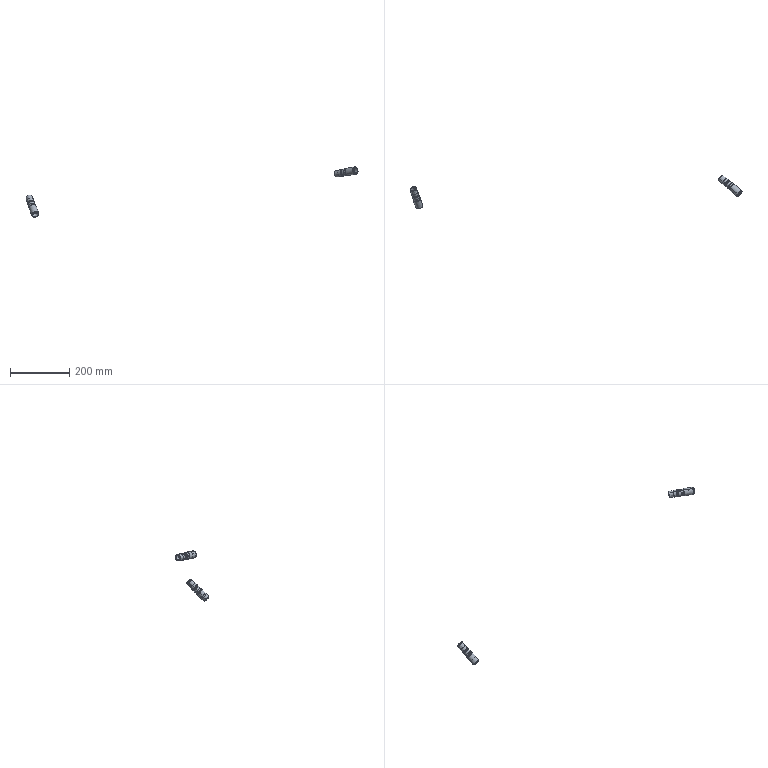Part | STEP file | TOCHA-1-SOLID1 | 2 solids | 8288 faces | volume 28159 mm3 | plane 7126 | cylinder 1114 | cone 28 | torus 20 | commonest cylinder face diameters 22.86 x1058 21.793 x16 22.606 x16 15.875 x4 17.069 x4 18.923 x4